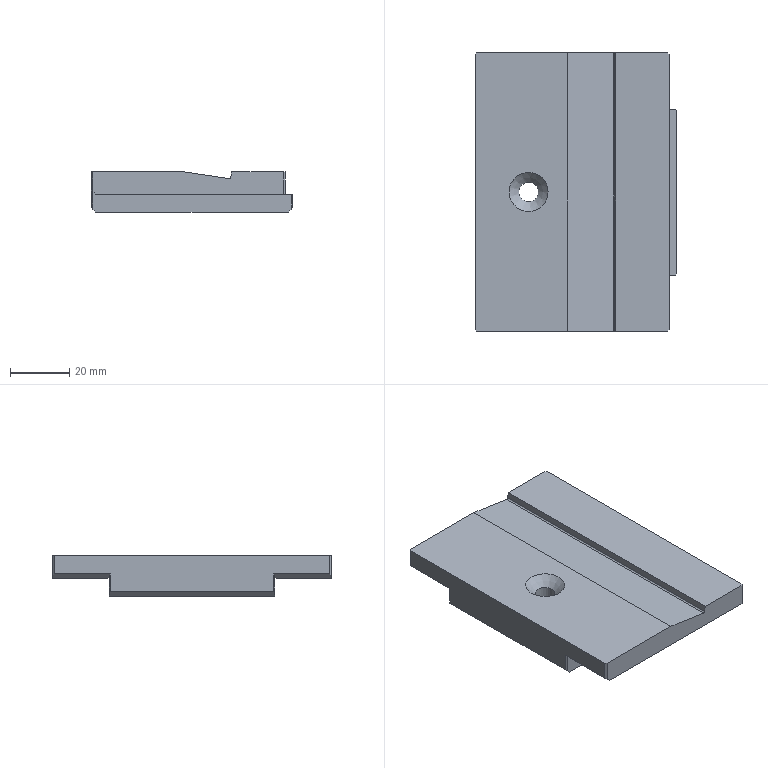NC program | NX | posted with a generic post | part box 68 x 94 x 13.65 mm
Lines 1 to 815 of 2371:
N10 G17 G21 G94 G90
(ADAPTIVE_MILLING_1 , TOOL : D12开粗)
N12 T02 M6
N14 G54
N16 G17 G0 G90 X-0.674 Y47.544 B0. C0. S6500 M3
N18 G43 Z30. H2
N20 Z-2.85
N22 G94 G1 X-0.68 Y47.394 Z-3.787 F3000.
N24 X-0.686 Y47.244 Z-4.158
N26 X-0.692 Y47.094 Z-4.43
N28 X-0.698 Y46.944 Z-4.65
N30 X-0.704 Y46.794 Z-4.834
N32 X-0.71 Y46.644 Z-4.992
N34 X-0.716 Y46.494 Z-5.13
N36 X-0.722 Y46.345 Z-5.25
N38 X-0.728 Y46.195 Z-5.355
N40 X-0.734 Y46.045 Z-5.448
N42 X-0.741 Y45.895 Z-5.529
N44 X-0.747 Y45.745 Z-5.6
N46 X-0.753 Y45.595 Z-5.66
N48 X-0.759 Y45.445 Z-5.712
N50 X-0.765 Y45.295 Z-5.755
N52 X-0.771 Y45.145 Z-5.789
N54 X-0.777 Y44.996 Z-5.816
N56 X-0.783 Y44.846 Z-5.835
N58 X-0.789 Y44.696 Z-5.846
N60 X-0.795 Y44.546 Z-5.85
N62 X-0.868 Y42.745
N64 G3 X0.013 Y41.529 R1.212
N66 X3.514 Y41.035 R14.844
N68 X13.481 Y40.902 R227.471
N70 G1 X18.066 Y40.9
N72 X46.55 Y40.898
N74 G2 X51.296 Y38.553 R6.652
N76 X53.66 Y33.706 R10.917
N78 X54.31 Y27.721 R31.183
N80 X54.399 Y14.852 R486.696
N82 G1 X54.398 Y-33.051
N84 G2 X52.084 Y-37.767 R6.642
N86 X47.306 Y-40.136 R10.815
N88 X41.503 Y-40.8 R29.773
N90 X28.094 Y-40.899 R451.076
N92 G1 X-46.583 Y-40.897
N94 G2 X-51.291 Y-38.57 R6.637
N96 X-53.628 Y-33.853 R10.808
N98 X-54.295 Y-28.14 R29.261
N100 X-54.399 Y-14.956 R420.423
N102 G1 X-54.398 Y33.055
N104 G2 X-52.057 Y37.803 R6.639
N106 X-47.199 Y40.165 R10.925
N108 X-41.168 Y40.813 R31.476
N110 X-28.524 Y40.899 R496.813
N112 G1 X23.391 Y40.897
N114 G3 X27.515 Y40.404 R19.277
N116 X37.552 Y40.301 R316.899
N118 G2 X44.389 Y40.282 R527.538
N120 X50.916 Y36.521 R8.631
N122 X53.115 Y31.047 R13.963
N124 X53.717 Y24.422 R41.238
N126 X53.799 Y11.282 R594.915
N128 G1 X53.797 Y-30.484
N130 G2 X50.052 Y-37.394 R8.604
N132 X44.585 Y-39.608 R13.899
N134 X37.691 Y-40.224 R42.056
N136 X24.641 Y-40.299 R651.935
N138 G1 X-44.003 Y-40.297
N140 G2 X-50.878 Y-36.581 R8.586
N142 X-53.096 Y-31.148 R13.824
N144 X-53.72 Y-24.345 R41.046
N146 X-53.799 Y-11.476 R610.363
N148 G1 X-53.797 Y30.503
N150 G2 X-50.114 Y37.354 R8.583
N152 X-44.604 Y39.606 R13.827
N154 X-37.844 Y40.22 R41.336
N156 X-23.978 Y40.299 R656.577
N158 G1 X23.392 Y40.297
N160 X24.461 Y40.15
N162 X27.501
N164 G3 X34.958 Y39.731 R63.624
N166 G2 X42.414 Y39.679 R748.413
N168 X50.465 Y34.845 R9.878
N170 X52.572 Y28.851 R16.456
N172 X53.126 Y21.723 R51.169
N174 X53.198 Y9.663 R694.236
N176 G1 X53.196 Y-28.279
N178 G2 X48.307 Y-36.989 R9.918
N180 X42.441 Y-39.056 R16.409
N182 X35.315 Y-39.624 R50.031
N184 G1 X29.826 Y-39.702
N186 X28.698 Y-40.032
N188 X27.499 Y-40.15
N190 X-27.501
N192 G3 X-35.1 Y-39.724 R60.239
N194 G2 X-42.386 Y-39.679 R721.319
N196 X-50.442 Y-34.884 R9.862
N198 X-52.55 Y-28.976 R16.287
N200 X-53.123 Y-21.85 R49.74
N202 X-53.198 Y-9.791 R649.321
N204 G1 X-53.196 Y28.253
N206 G2 X-48.375 Y36.948 R9.904
N208 X-42.509 Y39.045 R16.262
N210 X-35.429 Y39.621 R49.122
N212 G3 X-29.805 Y39.705 R765.749
N214 G1 X-28.698 Y40.032
N216 X-27.5 Y40.15
N218 X27.501
N220 X28.701 Y40.031
N222 G3 X32.73 Y39.308 R14.812
N224 X40.428 Y39.098 R159.407
N226 G2 X47.086 Y36.798 R11.004
N228 X51.018 Y31.06 R12.621
N230 X52.288 Y24.587 R25.785
N232 X52.581 Y15.459 R121.399
N234 G1 X52.598 Y6.459
N236 X52.597 Y-26.118
N238 G2 X51.737 Y-31.14 R12.756
N240 X46.39 Y-36.728 R11.156
N242 X40.066 Y-38.569 R19.654
N244 X32.017 Y-39.051 R69.857
N246 G3 X30.765 Y-39.198 R3.885
N248 G1 X29.852 Y-39.682
N250 X29.68 Y-39.734
N252 G3 X30.724 Y-39.217 R5.797
N254 G2 X32.317 Y-38.855 R4.748
N256 X37.759 Y-38.433 R603.695
N258 G3 X44.094 Y-37.153 R25.438
N260 X49.627 Y-33.281 R12.056
N262 X51.886 Y-27.571 R11.913
N264 X52.218 Y-21.42 R48.25
N266 G1 X52.237 Y-13.815
N268 X52.236 Y10.23
N270 G3 X52.064 Y22.153 R266.298
N272 X51.157 Y28.966 R34.371
N274 X48.271 Y34.729 R13.937
N276 X41.802 Y38.28 R11.099
N278 X36.653 Y38.758 R36.555
N280 G2 X31.134 Y39.169 R52.618
N282 X30.536 Y39.317 R3.054
N284 G3 X29.683 Y39.733 R4.424
N286 G2 X30.536 Y39.317 R4.424
N288 G3 X32.831 Y38.616 R6.855
N290 X37.929 Y38.106 R67.403
N292 G2 X42.773 Y37.161 R18.636
N294 X49.244 Y31.204 R11.752
N296 X51.077 Y24.831 R20.574
N298 X51.589 Y16.257 R72.007
N300 X51.637 Y4.107 R779.369
N302 G1 X51.636 Y-16.518
N304 G2 X51.48 Y-24.795 R133.04
N306 X50.316 Y-30.041 R15.405
N308 X44.567 Y-35.807 R11.806
N310 X38.408 Y-37.583 R20.973
N312 X33.119 Y-38.195 R297.497
N314 G3 X31.648 Y-38.538 R5.082
N316 G1 X30.915 Y-39.114
N318 X30.796 Y-39.178
N320 G3 X31.614 Y-38.542 R5.507
N322 G2 X33.519 Y-37.937 R5.886
N324 X38.424 Y-37.188 R738.211
N326 G3 X44.444 Y-35.264 R19.887
N328 X50.457 Y-27.502 R11.874
N330 X51.186 Y-21.618 R27.693
N332 X51.277 Y-10.414 R366.554
N334 G1 X51.275 Y7.916
N336 G3 X51.089 Y20.333 R265.82
N338 X50.134 Y27.366 R35.26
N340 X47.174 Y33.277 R14.55
N342 X40.893 Y37.047 R12.249
N344 X35.623 Y37.903 R36.581
N346 G2 X31.719 Y38.598 R21.819
N348 X30.918 Y39.113 R2.025
N350 G1 X30.799 Y39.176
N352 G2 X31.579 Y38.585 R8.011
N354 G3 X34.226 Y37.686 R8.572
N356 G2 X38.887 Y36.817 R264.531
N358 X44.63 Y34.235 R14.028
N360 X48.933 Y28.049 R13.694
N362 X50.309 Y21.322 R27.004
N364 X50.657 Y11.431 R120.082
N366 G1 X50.676 Y2.836
N368 X50.675 Y-13.199
N370 G2 X50.508 Y-22.286 R153.407
N372 X49.425 Y-27.971 R19.938
N374 X43.065 Y-34.795 R12.422
N376 X37.319 Y-36.603 R23.309
N378 G3 X33.194 Y-37.482 R50.092
N380 X32.311 Y-37.886 R2.329
N382 G2 X31.57 Y-38.577 R9.068
N384 G3 X32.412 Y-37.786 R9.652
N386 G2 X34.439 Y-36.949 R6.381
N388 G3 X39.038 Y-35.808 R401.807
N390 X44.797 Y-33.09 R16.95
N392 X49.367 Y-26.073 R12.825
N394 X50.204 Y-19.752 R28.871
N396 X50.316 Y-8.053 R327.252
N398 G1 X50.314 Y5.687
N400 G3 X50.132 Y18.329 R283.747
N402 X49.168 Y25.679 R37.688
N404 X46.162 Y31.861 R15.483
N406 X39.982 Y35.924 R13.365
N408 X34.999 Y37.158 R48.883
N410 G2 X32.209 Y38.037 R12.598
N412 G1 X31.467 Y38.662
N414 G2 X32.291 Y37.924 R15.573
N416 G3 X34.781 Y36.812 R8.411
N418 G2 X39.109 Y35.496 R92.052
N420 X47.741 Y27.118 R13.962
N422 X49.3 Y20.064 R26.562
N424 X49.691 Y10.22 R111.024
N426 G1 X49.716 Y-0.355
N428 X49.705 Y-13.825
N430 G2 X49.407 Y-21.736 R82.984
N432 X47.83 Y-27.757 R17.963
N434 X41.677 Y-33.814 R13.329
N436 X36.488 Y-35.72 R29.806
N438 G3 X33.263 Y-36.867 R18.507
N440 G1 X32.947 Y-37.119
N442 X32.348 Y-37.849
N444 G2 X33.164 Y-36.897 R8.535
N446 X35.489 Y-35.765 R8.702
N448 G3 X40.205 Y-34.012 R61.725
N450 X45.981 Y-29.561 R14.472
N452 X48.692 Y-23.081 R15.463
N454 X49.296 Y-16.05 R43.352
N456 X49.355 Y1.109 R954.366
N458 X49.212 Y15.598 R426.543
N460 X48.362 Y23.417 R45.593
N462 X45.602 Y29.97 R17.464
N464 X39.438 Y34.772 R14.397
N466 X34.979 Y36.374 R63.972
N468 G2 X32.736 Y37.407 R9.388
N470 G1 X32.158 Y38.039
N472 G2 X32.882 Y37.22 R41.672
N474 G3 X35.092 Y35.934 R8.401
N476 G2 X39.34 Y34.063 R69.517
N478 X46.898 Y25.375 R15.204
N480 X48.377 Y18.027 R29.53
N482 X48.737 Y7.416 R132.473
N484 G1 X48.755 Y-2.079
N486 G2 X48.666 Y-16.358 R534.947
N488 X47.955 Y-22.971 R35.777
N490 X43.845 Y-30.449 R14.32
N492 X38.533 Y-33.815 R18.559
N494 G3 X34.665 Y-35.497 R102.761
N496 X33.496 Y-36.258 R4.146
N498 X33.113 Y-36.918 R6.345
N500 G1 X32.998 Y-37.057
N502 G3 X33.464 Y-36.267 R4.36
N504 G2 X35.079 Y-35.082 R5.282
N506 X39.095 Y-33.125 R463.861
N508 G3 X44.493 Y-28.915 R16.551
N510 X47.624 Y-21.98 R15.934
N512 X48.309 Y-15.047 R40.777
N514 X48.394 Y-0.828 R575.144
N516 X48.241 Y14.11 R421.264
N518 X47.366 Y22.063 R46.714
N520 X44.467 Y28.943 R18.378
N522 X38.604 Y33.852 R16.247
N524 X34.688 Y35.755 R704.393
N526 G2 X33.286 Y36.664 R5.938
N528 G1 X33.176 Y36.806
N530 G2 X34.947 Y38.379 R1.2
N532 G1 X35.182 Y38.143 Z-5.836
N534 X35.401 Y37.893 Z-5.822
N536 X36.543 Y36.616 Z-5.75
N538 G3 X38.346 Y38.192 R1.2 F15000.
N540 G1 X38.108 Y38.508
N542 X37.857 Y38.815
N544 G3 X37.043 Y39.17 R1.203
N546 G1 X35.09 Y39.233
N548 X33.678 Y39.273 Z-5.809 F3000.
N550 G3 X32.824 Y38.881 Z-5.85 R1.2
N552 X32.786 Y37.315 R1.2
N554 G2 X33.322 Y36.562 R4.285
N556 G3 X35.246 Y35.07 R7.242
N558 G2 X39.292 Y32.686 R79.527
N560 X46.07 Y23.645 R16.75
N562 X47.449 Y16.091 R32.861
N564 X47.776 Y5.613 R146.465
N566 X47.731 Y-13.556 R933.703
N568 X47.129 Y-20.724 R46.218
N570 X44.263 Y-27.665 R16.447
N572 X39.136 Y-32.142 R17.349
N574 G1 X35.268 Y-34.336
N576 G3 X33.888 Y-35.398 R5.468
N578 G1 X33.738 Y-35.674
N580 G3 X33.902 Y-36.793 R1.201
N582 X34.303 Y-37.164 Z-5.827 R1.963
N584 G1 X35.739 Y-38.299 Z-5.75
N586 X36.496 Y-38.897 F15000.
N588 G3 X38.373 Y-38.35 R1.2
N590 G1 X38.511 Y-37.961
N592 X38.633 Y-37.567
N594 G3 X36.61 Y-36.484 R1.2
N596 G1 X35.27 Y-37.809 Z-5.829 F3000.
N598 G2 X34.845 Y-38.053 Z-5.85 R1.22
N600 X33.419 Y-36.345 R1.2
N602 G3 X33.792 Y-35.513 R3.161
N604 G2 X35.079 Y-34.247 R4.319
N606 X38.506 Y-32.09 R75.318
N608 G3 X43.558 Y-27.676 R18.666
N610 X46.675 Y-20.404 R17.227
N612 X47.353 Y-13.108 R44.925
N614 X47.328 Y11.1 R706.972
N616 X46.583 Y19.745 R59.538
N618 X44.081 Y26.884 R21.333
N620 X38.45 Y32.642 R17.697
N622 G2 X34.806 Y34.967 R294.359
N624 X33.585 Y36.035 R5.011
N626 G1 X33.24 Y36.68
N628 G3 X34.175 Y35.217 R5.814
N630 X36.422 Y33.385 R16.836
N632 G2 X40.735 Y29.857 R30.76
N634 X45.424 Y21.312 R19.033
N636 X46.584 Y13.219 R40.872
N638 X46.827 Y0.938 R230.264
N640 X46.725 Y-13.281 R435.929
N642 X45.912 Y-20.469 R38.28
N644 X39.664 Y-30.265 R16.794
N646 X35.747 Y-33.079 R117.242
N648 G3 X34.117 Y-34.562 R7.747
N650 X33.738 Y-35.666 R5.903
N652 G2 X34.124 Y-34.502 R8.031
N654 X35.881 Y-32.699 R7.477
N656 G3 X39.639 Y-29.752 R108.589
N658 X45.565 Y-19.71 R17.698
N660 X46.367 Y-12.203 R42.131
N662 X46.335 Y10.52 R493.232
N664 X45.497 Y19.065 R55.277
N666 X42.566 Y26.713 R21.627
N668 X37.708 Y31.881 R21.453
N670 G2 X34.636 Y34.395 R47.676
N672 X33.818 Y35.41 R3.434
N674 G1 X33.682 Y35.852
N676 G3 X34.775 Y33.903 R4.021
N678 X37.729 Y31.127 R46.959
N680 G2 X42.913 Y24.396 R21.902
N682 X45.185 Y16.418 R26.756
N684 X45.797 Y7.083 R80.373
N686 X45.759 Y-11.77 R438.829
N688 X44.943 Y-19.14 R40.784
N690 X39.165 Y-29.076 R18.535
N692 X35.633 Y-32.155 R409.623
N694 G3 X34.177 Y-33.847 R6.961
N696 X34.031 Y-34.701 R2.642
N698 G2 X34.227 Y-33.66 R2.81
N700 X35.88 Y-31.618 R8.137
N702 G3 X39.426 Y-28.254 R118.421
N704 X44.682 Y-18.019 R19.591
N706 X45.409 Y-10.548 R47.004
N708 X45.334 Y10.059 R371.62
N710 X44.36 Y18.679 R51.13
N712 X39.859 Y28.218 R21.919
N714 X36.1 Y32.091 R46.509
N716 G2 X34.149 Y34.339 R12.184
N718 G1 X34.042 Y34.635
N720 G2 X35.82 Y35.882 R1.2
N722 X36.334 Y35.309 Z-5.817 R1.304
N724 G1 X37.093 Y33.904 Z-5.75
N726 G3 X37.507 Y33.354 R1.536 F15000.
N728 X39.394 Y34.635 R1.2
N730 G1 X39.288 Y35.01
N732 X39.169 Y35.381
N734 G3 X38.331 Y36.069 R1.201
N736 G1 X36.637 Y36.447
N738 X35.919 Y36.609 Z-5.781 F3000.
N740 X35.199 Y36.761 Z-5.812
N742 G3 X34.337 Y36.564 Z-5.85 R1.2
N744 X33.871 Y35.229 R1.2
N746 G2 X34.102 Y34.303 R7.454
N748 G3 X35.465 Y32.211 R7.359
N750 G2 X38.743 Y28.512 R217.642
N752 X43.788 Y17.742 R24.009
N754 X44.734 Y8.983 R55.23
N756 X44.777 Y-10.769 R318.394
N758 X43.859 Y-18.397 R40.093
N760 X38.693 Y-27.879 R20.536
N762 G3 X35.432 Y-31.274 R380.167
N764 X34.223 Y-32.979 R7.321
N766 X34.15 Y-33.501 R1.907
N768 G1 X34.092 Y-34.083
N770 G3 X34.155 Y-33.151 R16.277
N772 G2 X34.998 Y-31.516 R4.417
N774 X37.716 Y-28.407 R42.878
N776 G3 X41.976 Y-22.292 R24.386
N778 X44.081 Y-14.415 R25.327
N780 X44.517 Y-5.565 R84.713
N782 X44.315 Y9.867 R271.895
N784 X43.199 Y18.422 R47.469
N786 X37.73 Y29.027 R24.799
N788 G2 X34.898 Y32.442 R63.949
N790 X34.121 Y33.857 R4.812
N792 G1 X34.046 Y34.56
N794 G3 X34.281 Y33.149 R5.054
N796 X35.875 Y30.531 R11.714
N798 G2 X39.215 Y25.924 R65.74
N800 X43.002 Y15.723 R27.549
N802 X43.818 Y6.452 R67.415
N804 X43.77 Y-10.285 R240.551
N806 X42.684 Y-18.07 R37.703
N808 X38.191 Y-26.715 R23.017
N810 G3 X35.241 Y-30.328 R164.642
N812 X34.189 Y-32.127 R7.19
N814 X34.15 Y-33.243 R5.881
N816 G2 X34.182 Y-32.042 R7.159
N818 X35.408 Y-29.734 R7.464
N820 G3 X38.501 Y-25.666 R917.804
N822 X42.92 Y-14.647 R24.47
N824 X43.523 Y-6.124 R65.041
N826 X43.299 Y9.53 R214.851
N828 X42.002 Y18.332 R45.335
N830 X37.326 Y27.921 R28.43
N832 G2 X34.844 Y31.484 R55.747
N834 X34.158 Y33.02 R5.002
N836 G1 X34.132 Y33.678
N838 G3 X34.182 Y32.62 R17.964
N840 X35.31 Y30.058 R8.489
N842 G2 X38.097 Y25.64 R554.332
N844 X42.147 Y14.021 R31.162
N846 X42.892 Y3.796 R80.905
N848 X42.75 Y-9.925 R177.116
N850 X41.445 Y-17.992 R35.826
N852 X37.501 Y-25.807 R26.589
N854 G3 X34.855 Y-29.614 R72.033
N856 X34.166 Y-31.076 R5.536
N858 G1 X34.15 Y-32.336
N860 G2 X34.177 Y-30.903 R11.57
N862 X35.286 Y-28.512 R8.221
N864 G3 X38.21 Y-24.034 R369.87
N866 X42.035 Y-12.968 R27.473
N868 X42.571 Y-3.494 R78.291
N870 X42.227 Y9.863 R157.151
N872 X40.558 Y19.098 R41.57
N874 X36.727 Y27.086 R34.5
N876 G2 X34.582 Y30.794 R37.488
N878 X34.15 Y32.063 R4.514
N880 G1 Y32.918
N882 G3 X34.224 Y31.264 R7.853
N884 X35.537 Y28.157 R12.99
N886 G2 X38.39 Y22.732 R87.484
N888 X41.371 Y11.647 R36.519
N890 X41.96 Y0.103 R106.566
N892 X41.616 Y-10.822 R108.143
N894 X39.422 Y-20.027 R30.998
N896 X36.539 Y-25.381 R37.416
N898 G3 X34.386 Y-29.118 R32.289
N900 X34.15 Y-29.891 R2.31
N902 G1 Y-31.151
N904 G2 X34.176 Y-29.543 R14.275
N906 X35.281 Y-26.927 R10.009
N908 G3 X38.031 Y-22.018 R134.723
N910 X41.157 Y-11.172 R31.072
N912 X41.593 Y-0.477 R94.351
N914 X41.028 Y11.204 R107.266
N916 X36.535 Y25.513 R37.533
N918 G2 X34.466 Y29.693 R42.752
N920 X34.15 Y30.766 R5.032
N922 G1 Y31.801
N924 G3 X34.197 Y30.004 R12.488
N926 X35.3 Y26.882 R13.692
N928 G2 X37.89 Y21.127 R104.559
N930 X40.513 Y9.717 R42.111
N932 X40.717 Y-8.938 R120.404
N934 X38.769 Y-18.475 R35.496
N936 X35.977 Y-24.388 R43.051
N938 G3 X34.203 Y-28.038 R26.917
N940 G1 X34.15 Y-28.347
N942 Y-29.787
N944 G2 X34.169 Y-28.041 R32.747
N946 X35.123 Y-25.431 R10.695
N948 G3 X37.672 Y-20.112 R117.675
N950 X40.274 Y-9.304 R35.398
N952 X40.515 Y3.826 R108.206
N954 X39.407 Y14.466 R65.655
N956 X36.026 Y24.419 R43.825
N958 G2 X34.297 Y28.59 R37.057
N960 X34.15 Y29.215 R8.524
N962 G1 Y30.43
N964 G3 X34.19 Y28.4 R16.352
N966 X35.298 Y24.846 R17.17
N968 G2 X37.785 Y18.113 R76.268
N970 X39.707 Y6.914 R51.384
N972 X39.68 Y-8.641 R104.804
N974 X36.031 Y-22.073 R37.357
N976 G3 X34.211 Y-26.25 R44.793
N978 G1 X34.15 Y-26.575
N980 Y-28.24
N982 G2 X34.167 Y-26.271 R135.856
N984 X35.062 Y-23.508 R12.672
N986 G3 X37.476 Y-17.46 R81.204
N988 X39.411 Y-6.91 R41.688
N990 X38.976 Y10.387 R97.734
N992 X35.8 Y22.55 R48.678
N994 G2 X34.237 Y26.952 R44.754
N996 G1 X34.15 Y27.4
N998 Y28.84
N1000 G3 X34.187 Y26.451 R24.712
N1002 X35.186 Y22.734 R21.366
N1004 G2 X37.553 Y14.697 R71.381
N1006 X38.902 Y2.73 R66.716
N1008 X38.515 Y-9.493 R82.259
N1010 X35.624 Y-20.474 R41.622
N1012 G3 X34.169 Y-24.38 R44.156
N1014 X34.15 Y-26.479 R36.536
N1016 G1 X34.164 Y-24.232
N1018 G2 X35.079 Y-21.04 R16.56
N1020 G3 X37.386 Y-13.622 R59.154
N1022 X38.552 Y-3.083 R54.019
N1024 X37.79 Y11.19 R84.905
N1026 X35.309 Y21.18 R58.764
N1028 G2 X34.151 Y25.193 R34.115
N1030 G1 X34.15 Y26.875
N1032 G3 X34.18 Y24.15 R35.162
N1034 X35.08 Y20.163 R27.778
N1036 G2 X37.439 Y8.795 R68.347
N1038 X37.563 Y-8.409 R82.194
N1040 X35.058 Y-19.172 R48.538
N1042 G3 X34.155 Y-22.089 R32.037
N1044 G1 X34.15 Y-24.45
N1046 X34.163 Y-21.801
N1048 G2 X35. Y-18.344 R22.005
N1050 G3 X37.546 Y-2.148 R54.737
N1052 X36.437 Y12.861 R76.226
N1054 X34.561 Y20.716 R108.581
N1056 G2 X34.15 Y22.571 R46.063
N1058 G1 Y24.551
N1060 G3 X34.175 Y21.28 R58.798
N1062 X34.862 Y17.432 R35.665
N1064 G2 X36.56 Y-7.783 R77.504
N1066 X34.806 Y-16.691 R55.034
N1068 G3 X34.15 Y-19.28 R27.084
N1070 G1 Y-21.98
N1072 G2 X34.173 Y-18.707 R56.918
N1074 X34.972 Y-14.678 R40.152
N1076 G3 X36.516 Y1.133 R62.745
N1078 X34.721 Y16.304 R77.03
N1080 G2 X34.15 Y19.264 R191.017
N1082 G1 Y21.694
N1084 G3 X34.179 Y17.416 R84.762
N1086 X34.941 Y11.948 R93.591
N1088 G2 X35.886 Y-0.245 R82.959
N1090 G1 X35.887 Y-15.11
N1092 G3 X36.031 Y-15.68 R1.218
N1094 X36.907 Y-16.302 Z-5.803 R1.257
N1096 G1 X38.137 Y-16.61 Z-5.75
N1098 X39.136 Y-16.86 F15000.
N1100 G2 X39.671 Y-18.894 R1.2
N1102 X39.259 Y-19.233 R1.926
N1104 G1 X39.122 Y-19.296
N1106 X38.979 Y-19.346
N1108 X37.139 Y-19.827
N1110 X36.357 Y-20.035 Z-5.784 F3000.
N1112 X35.571 Y-20.231 Z-5.818
N1114 G2 X34.831 Y-20.137 Z-5.85 R1.201
N1116 X34.15 Y-19.055 R1.201
N1118 X34.537 Y-15.273 R16.274
N1120 G3 X35.303 Y-10.76 R52.023
N1122 X35.518 Y-3.835 R80.65
N1124 G1 X35.523 Y-1.765
N1126 Y14.585
N1128 G2 X35.628 Y15.074 R1.244
N1130 G1 X36.149 Y16.241
N1132 X37.12 Y18.412 Z-5.75
N1134 G2 X39.308 Y18.369 R1.2 F15000.
N1136 G1 X39.44 Y18.067
N1138 X39.556 Y17.758
N1140 G2 X37.361 Y16.84 R1.2
N1142 G1 X37.136 Y17.228
N1144 X36.347 Y18.578 Z-5.816 F3000.
N1146 G3 X35.709 Y19.059 Z-5.85 R1.201
N1148 X34.15 Y17.914 R1.2
N1150 X34.204 Y14.044 R52.26
N1152 G2 X34.738 Y8.621 R661.323
N1154 X34.918 Y-1.321 R171.833
N1156 G1 Y-14.251
N1158 G3 X35.159 Y-14.973 R1.206
N1160 G1 X35.692 Y-15.681
N1162 X37.123 Y-17.582 Z-5.75
N1164 X37.921 Y-18.642 F15000.
N1166 G3 X39.553 Y-16.927 R-1.2
N1168 G1 X39.367 Y-16.803
N1170 X39.176 Y-16.686
N1172 G3 X37.687 Y-17.042 R1.2
N1174 G1 X37.139 Y-17.772
N1176 X36.701 Y-18.358 Z-5.781 F3000.
N1178 X36.255 Y-18.938 Z-5.812
N1180 G2 X35.464 Y-19.349 Z-5.85 R1.2
N1182 X34.15 Y-18.155 R1.2
N1184 X34.353 Y-14.634 R22.477
N1186 G3 X34.541 Y-8.159 R78.567
N1188 G1 X34.556 Y-2.939
N1190 X34.557 Y11.656
N1192 G2 X35.023 Y12.605 R1.201
N1194 X36.504 Y12.595 Z-5.783 R1.205
N1196 G1 X37.117 Y12.107 Z-5.75
N1198 X38.007 Y11.399 F15000.
N1200 G3 X39.726 Y13.041 R1.2
N1202 G1 X39.485 Y13.378
N1204 X39.235 Y13.708
N1206 X39.137 Y13.8
N1208 X39.033 Y13.885
N1210 X37.141 Y15.204
N1212 X35.973 Y16.012 Z-5.81 F3000.
N1214 G3 X35.051 Y16.151 Z-5.85 R1.2
N1216 X34.15 Y14.989 R1.2
N1218 G1 Y-16.871
N1220 G3 X34.69 Y-17.874 R1.201
N1222 G1 X35.134 Y-18.166
N1224 X37.121 Y-19.474 Z-5.75
N1226 X37.328 Y-19.61 F15000.
N1228 X37.529 Y-19.756
N1230 G2 X37.935 Y-20.656 R1.202
N1232 G1 Y-34.037
N1234 G2 X37.167 Y-37.348 R7.74
N1236 X35.883 Y-39.443 R11.033
N1238 G1 X35.316 Y-40.176
N1240 X34.737 Y-40.899
N1242 G2 X32.359 Y-42.66 R6.879
N1244 X29.944 Y-43.358 R8.516
N1246 X24.783 Y-43.754 R36.475
N1248 G1 X-24.917 Y-43.816
N1250 G2 X-25.869 Y-43.347 R1.201
N1252 G1 X-26.032 Y-43.136
N1254 X-27.482 Y-41.25 Z-5.85 F3000.
N1256 X-27.833 Y-40.788
N1258 X-28.196 Y-40.336
N1260 G3 X-28.701 Y-40.031 R1.217
N1262 X-32.824 Y-39.295 R14.996
N1264 X-40.399 Y-39.097 R159.428
N1266 G2 X-46.98 Y-36.883 R11.018
N1268 X-50.969 Y-31.195 R12.507
N1270 X-52.276 Y-24.73 R25.239
N1272 X-52.584 Y-15.063 R122.752
N1274 G1 X-52.597 Y-7.548
N1276 Y26.138
N1278 G2 X-51.713 Y31.2 R12.685
N1280 X-46.374 Y36.737 R11.163
N1282 X-40.268 Y38.541 R19.457
N1284 X-32.271 Y39.044 R65.396
N1286 G3 X-30.839 Y39.169 R5.763
N1288 G1 X-29.852 Y39.682
N1290 X-29.68 Y39.734
N1292 G3 X-30.718 Y39.22 R5.756
N1294 G2 X-32.166 Y38.873 R4.286
N1296 X-37.553 Y38.452 R254.594
N1298 G3 X-43.899 Y37.224 R26.386
N1300 X-49.403 Y33.563 R12.281
N1302 X-51.845 Y27.841 R11.595
N1304 X-52.207 Y22.277 R40.399
N1306 G1 X-52.237 Y13.863
N1308 X-52.235 Y-10.317
N1310 G3 X-52.047 Y-22.465 R248.388
N1312 X-51.064 Y-29.311 R32.375
N1314 X-48.008 Y-35.02 R13.492
N1316 X-41.75 Y-38.288 R11.157
N1318 X-36.601 Y-38.756 R37.214
N1320 G2 X-31.124 Y-39.166 R50.455
N1322 X-30.544 Y-39.313 R3.088
N1324 G3 X-29.683 Y-39.733 R4.479
N1326 G2 X-30.544 Y-39.313 R4.479
N1328 G3 X-32.743 Y-38.625 R6.576
N1330 X-37.945 Y-38.101 R66.781
N1332 G2 X-42.832 Y-37.138 R18.433
N1334 X-49.251 Y-31.189 R11.754
N1336 X-51.092 Y-24.721 R20.751
N1338 X-51.588 Y-16.37 R72.122
N1340 X-51.637 Y-4.176 R776.556
N1342 G1 X-51.635 Y16.539
N1344 G2 X-51.478 Y24.816 R132.008
N1346 X-50.381 Y29.894 R15.553
N1348 X-44.565 Y35.809 R11.782
N1350 X-38.27 Y37.603 R21.205
N1352 X-33.098 Y38.198 R409.229
N1354 G3 X-31.634 Y38.545 R4.86
N1356 G1 X-30.836 Y39.157
N1358 G3 X-31.624 Y38.534 R23.598
N1360 G2 X-33.532 Y37.934 R6.015
N1362 X-38.486 Y37.176 R859.981
N1364 G3 X-44.538 Y35.215 R19.649
N1366 X-50.483 Y27.402 R11.895
N1368 X-51.194 Y21.38 R28.785
N1370 X-51.277 Y10.851 R385.571
N1372 G1 X-51.275 Y-7.974
N1374 G3 X-51.086 Y-20.391 R261.649
N1376 X-50.095 Y-27.51 R34.622
N1378 X-47.044 Y-33.423 R14.339
N1380 X-40.798 Y-37.07 R12.325
N1382 X-36.364 Y-37.813 R32.635
N1384 G2 X-32.032 Y-38.499 R29.894
N1386 X-30.918 Y-39.113 R2.25
N1388 G1 X-30.839 Y-39.155
N1390 X-31.59 Y-38.577
N1392 G3 X-34.163 Y-37.695 R8.408
N1394 G2 X-38.816 Y-36.83 R407.126
N1396 X-44.583 Y-34.268 R14.127
N1398 X-48.919 Y-28.084 R13.657
N1400 X-50.326 Y-21.135 R27.276
N1402 X-50.657 Y-11.423 R123.432
N1404 G1 X-50.676 Y-2.738
N1406 X-50.675 Y13.387
N1408 G2 X-50.494 Y22.473 R142.649
N1410 X-49.376 Y28.102 R19.318
N1412 X-43.053 Y34.801 R12.427
N1414 X-37.356 Y36.596 R23.268
N1416 G3 X-33.206 Y37.478 R51.682
N1418 X-32.306 Y37.892 R2.317
N1420 G2 X-31.57 Y38.577 R9.057
N1422 G3 X-32.412 Y37.786 R9.692
N1424 G2 X-34.426 Y36.952 R6.332
N1426 G3 X-39.098 Y35.791 R342.908
N1428 X-44.801 Y33.088 R16.865
N1430 X-49.377 Y26.04 R12.83
N1432 X-50.196 Y19.942 R28.512
N1434 X-50.316 Y8.558 R293.299
N1436 G1 X-50.314 Y-5.677
N1438 G3 X-50.132 Y-18.319 R283.788
N1440 X-49.191 Y-25.583 R38.072
N1442 X-46.164 Y-31.856 R15.55
N1444 X-39.947 Y-35.932 R13.373
N1446 X-35.056 Y-37.141 R47.778
N1448 G2 X-32.222 Y-38.027 R12.902
N1450 X-31.467 Y-38.662 R38.573
N1452 X-32.297 Y-37.919 R16.129
N1454 G3 X-34.619 Y-36.86 R8.001
N1456 G2 X-38.913 Y-35.563 R136.442
N1458 X-45.247 Y-31.365 R14.185
N1460 X-48.479 Y-24.838 R16.384
N1462 X-49.499 Y-17.495 R37.556
N1464 X-49.712 Y-5.304 R241.594
N1466 G1 X-49.715 Y0.231
N1468 X-49.705 Y13.791
N1470 G2 X-49.406 Y21.747 R83.008
N1472 X-47.846 Y27.726 R17.963
N1474 X-41.655 Y33.826 R13.333
N1476 X-36.937 Y35.587 R27.892
N1478 G3 X-33.483 Y36.756 R25.141
N1480 X-32.944 Y37.124 R1.747
N1482 G1 X-32.348 Y37.849
N1484 G2 X-33.161 Y36.9 R8.872
N1486 X-35.542 Y35.746 R8.86
N1488 G3 X-40.141 Y34.041 R62.088
N1490 X-45.903 Y29.665 R14.555
N1492 X-48.666 Y23.215 R15.303
N1494 X-49.286 Y16.412 R41.253
N1496 X-49.355 Y-1.153 R912.259
N1498 X-49.21 Y-15.641 R420.726
N1500 X-48.38 Y-23.327 R45.805
N1502 X-45.734 Y-29.781 R17.693
N1504 X-39.377 Y-34.795 R14.385
N1506 X-34.841 Y-36.421 R74.169
N1508 G2 X-32.737 Y-37.405 R9.064
N1510 G1 X-32.179 Y-38.019
N1512 X-32.878 Y-37.222
N1514 G3 X-35.287 Y-35.845 R8.86
N1516 G2 X-39.628 Y-33.908 R52.548
N1518 X-46.844 Y-25.517 R15.124
N1520 X-48.358 Y-18.222 R28.852
N1522 X-48.733 Y-7.972 R123.323
N1524 G1 X-48.755 Y2.018
N1526 G2 X-48.666 Y16.342 R540.34
N1528 X-47.94 Y23.043 R35.619
N1530 X-43.64 Y30.638 R14.257
N1532 X-38.27 Y33.931 R19.287
N1534 G3 X-34.509 Y35.578 R66.353
N1536 X-33.441 Y36.327 R3.194
N1538 G2 X-32.998 Y37.057 R5.021
N1540 G3 X-33.464 Y36.268 R4.363
N1542 G2 X-35.092 Y35.075 R5.299
N1544 X-39.079 Y33.133 R505.431
N1546 G3 X-44.42 Y29.005 R16.64
N1548 X-47.58 Y22.188 R15.756
N1550 X-48.309 Y15.035 R39.969
N1552 X-48.394 Y0.816 R578.447
N1554 X-48.241 Y-14.122 R420.614
N1556 X-47.382 Y-21.986 R47.006
N1558 X-44.512 Y-28.878 R18.49
N1560 X-38.674 Y-33.812 R16.144
N1562 X-34.741 Y-35.724 R409.085
N1564 G2 X-33.284 Y-36.665 R5.921
N1566 G1 X-33.201 Y-36.771
N1568 G2 X-33.002 Y-37.588 R1.204
N1570 G1 X-33.118 Y-38.558
N1572 X-33.4 Y-40.92 Z-5.75
N1574 X-33.448 Y-41.406 F15000.
N1576 G3 X-33.201 Y-42.123 R1.206
N1578 G1 X-32.946 Y-42.46
N1580 X-32.679 Y-42.788
N1582 G3 X-30.78 Y-42.52 R1.2
N1584 X-30.8 Y-41.314 Z-5.803 R1.243 F3000.
N1586 G1 X-31.29 Y-40.309 Z-5.85
N1588 X-32.633 Y-37.552
N1590 G3 X-33.12 Y-36.906 R6.801
N1592 X-34.174 Y-35.772 R3.101
N1594 X-37.504 Y-33.784 R36.733
N1596 G2 X-42.701 Y-29.719 R19.325
N1598 X-46.44 Y-22.391 R18.022
N1600 X-47.555 Y-14.563 R39.55
N1602 X-47.788 Y-2.372 R231.231
N1604 X-47.715 Y14.143 R709.822
N1606 X-47.042 Y21.167 R41.535
N1608 X-43.614 Y28.478 R15.818
N1610 X-38.553 Y32.487 R18.971
N1612 G3 X-34.889 Y34.579 R80.477
N1614 X-33.864 Y35.432 R3.913
N1616 G1 X-33.739 Y35.671
N1618 G3 X-33.902 Y36.793 R1.201
N1620 X-34.303 Y37.164 Z-5.827 R1.959
N1622 G1 X-35.74 Y38.297 Z-5.75
N1624 X-36.498 Y38.895 F15000.
N1626 G3 X-38.374 Y38.347 R1.2
N1628 G1 X-38.512 Y37.96